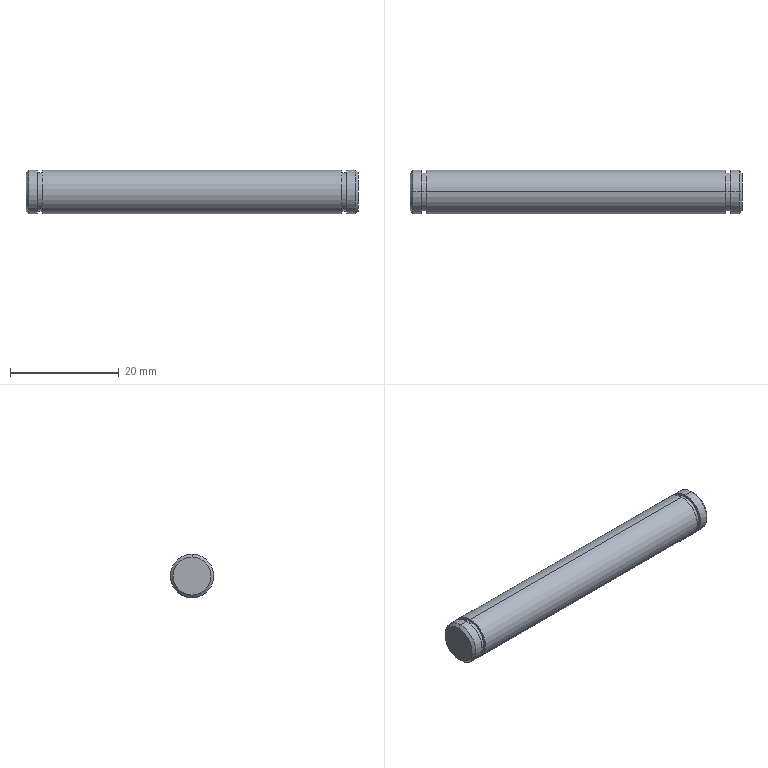Part | STEP file | 0217_Z_SCCG8-55-1 | 1 solid | 20 faces | box 61 x 8 x 8 mm | volume 3039 mm3 | cylinder 10 | plane 6 | cone 4 | commonest cylinder face diameters 8 x6 7 x4
STEP:
#1=CARTESIAN_POINT('',(0.,0.,0.));
#2=DIRECTION('',(0.,0.,1.));
#3=DIRECTION('',(1.,0.,0.));
#4=AXIS2_PLACEMENT_3D('',#1,#2,#3);
#5=CARTESIAN_POINT('',(3.,0.,-4.));
#6=VERTEX_POINT('',#5);
#7=CARTESIAN_POINT('',(3.,0.,4.));
#8=VERTEX_POINT('',#7);
#9=CARTESIAN_POINT('',(3.,0.,0.));
#10=DIRECTION('',(1.,0.,0.));
#11=DIRECTION('',(0.,0.,-1.));
#12=AXIS2_PLACEMENT_3D('',#9,#10,#11);
#13=CIRCLE('',#12,4.);
#14=CARTESIAN_POINT('',(30.5,0.,0.));
#15=DIRECTION('',(1.,0.,0.));
#16=DIRECTION('',(0.,0.,-1.));
#17=AXIS2_PLACEMENT_3D('',#14,#15,#16);
#18=CYLINDRICAL_SURFACE('',#17,4.);
#19=CARTESIAN_POINT('',(0.,-27.5));
#20=DIRECTION('',(1.,0.));
#21=VECTOR('',#20,1.);
#22=LINE('',#19,#21);
#23=(GEOMETRIC_REPRESENTATION_CONTEXT(2)PARAMETRIC_REPRESENTATION_CONTEXT()REPRESENTATION_CONTEXT('',''));
#24=DEFINITIONAL_REPRESENTATION('',(#22),#23);
#25=PCURVE('',#18,#24);
#26=CARTESIAN_POINT('',(3.,3.75,0.));
#27=DIRECTION('',(-1.,0.,0.));
#28=DIRECTION('',(0.,0.,1.));
#29=AXIS2_PLACEMENT_3D('',#26,#27,#28);
#30=PLANE('',#29);
#31=CARTESIAN_POINT('',(-4.,-3.75));
#32=CARTESIAN_POINT('',(-4.,3.178));
#33=CARTESIAN_POINT('',(2.,-0.2859));
#34=CARTESIAN_POINT('',(8.,-3.75));
#35=CARTESIAN_POINT('',(2.,-7.214));
#36=CARTESIAN_POINT('',(-4.,-10.678));
#37=CARTESIAN_POINT('',(-4.,-3.75));
#38=(BOUNDED_CURVE()B_SPLINE_CURVE(2,(#31,#32,#33,#34,#35,#36,#37),.UNSPECIFIED.,.T.,.F.)B_SPLINE_CURVE_WITH_KNOTS((1,2,2,2,2,1),(-2.094,0.,2.094,4.189,6.283,8.378),.UNSPECIFIED.)CURVE()GEOMETRIC_REPRESENTATION_ITEM()RATIONAL_B_SPLINE_CURVE((1.,0.5,1.,0.5,1.,0.5,1.))REPRESENTATION_ITEM(''));
#39=(GEOMETRIC_REPRESENTATION_CONTEXT(2)PARAMETRIC_REPRESENTATION_CONTEXT()REPRESENTATION_CONTEXT('',''));
#40=DEFINITIONAL_REPRESENTATION('',(#38),#39);
#41=PCURVE('',#30,#40);
#42=SURFACE_CURVE('',#13,(#25,#41),.PCURVE_S1.);
#43=EDGE_CURVE('',#6,#8,#42,.T.);
#44=ORIENTED_EDGE('',*,*,#43,.T.);
#45=CARTESIAN_POINT('',(58.,0.,4.));
#46=VERTEX_POINT('',#45);
#47=CARTESIAN_POINT('',(30.5,0.,4.));
#48=DIRECTION('',(1.,0.,0.));
#49=VECTOR('',#48,1.);
#50=LINE('',#47,#49);
#51=CARTESIAN_POINT('',(3.142,0.));
#52=DIRECTION('',(0.,1.));
#53=VECTOR('',#52,1.);
#54=LINE('',#51,#53);
#55=(GEOMETRIC_REPRESENTATION_CONTEXT(2)PARAMETRIC_REPRESENTATION_CONTEXT()REPRESENTATION_CONTEXT('',''));
#56=DEFINITIONAL_REPRESENTATION('',(#54),#55);
#57=PCURVE('',#18,#56);
#58=CARTESIAN_POINT('',(30.5,0.,0.));
#59=DIRECTION('',(1.,0.,0.));
#60=DIRECTION('',(0.,0.,-1.));
#61=AXIS2_PLACEMENT_3D('',#58,#59,#60);
#62=CYLINDRICAL_SURFACE('',#61,4.);
#63=CARTESIAN_POINT('',(3.142,0.));
#64=DIRECTION('',(0.,1.));
#65=VECTOR('',#64,1.);
#66=LINE('',#63,#65);
#67=(GEOMETRIC_REPRESENTATION_CONTEXT(2)PARAMETRIC_REPRESENTATION_CONTEXT()REPRESENTATION_CONTEXT('',''));
#68=DEFINITIONAL_REPRESENTATION('',(#66),#67);
#69=PCURVE('',#62,#68);
#70=SURFACE_CURVE('',#50,(#57,#69),.PCURVE_S1.);
#71=EDGE_CURVE('',#8,#46,#70,.T.);
#72=ORIENTED_EDGE('',*,*,#71,.T.);
#73=CARTESIAN_POINT('',(58.,0.,-4.));
#74=VERTEX_POINT('',#73);
#75=CARTESIAN_POINT('',(58.,0.,0.));
#76=DIRECTION('',(-1.,0.,0.));
#77=DIRECTION('',(0.,0.,-1.));
#78=AXIS2_PLACEMENT_3D('',#75,#76,#77);
#79=CIRCLE('',#78,4.);
#80=CARTESIAN_POINT('',(6.283,27.5));
#81=DIRECTION('',(-1.,0.));
#82=VECTOR('',#81,1.);
#83=LINE('',#80,#82);
#84=(GEOMETRIC_REPRESENTATION_CONTEXT(2)PARAMETRIC_REPRESENTATION_CONTEXT()REPRESENTATION_CONTEXT('',''));
#85=DEFINITIONAL_REPRESENTATION('',(#83),#84);
#86=PCURVE('',#18,#85);
#87=CARTESIAN_POINT('',(58.,3.75,0.));
#88=DIRECTION('',(1.,0.,0.));
#89=DIRECTION('',(0.,0.,-1.));
#90=AXIS2_PLACEMENT_3D('',#87,#88,#89);
#91=PLANE('',#90);
#92=CARTESIAN_POINT('',(4.,-3.75));
#93=CARTESIAN_POINT('',(4.,-10.678));
#94=CARTESIAN_POINT('',(-2.,-7.214));
#95=CARTESIAN_POINT('',(-8.,-3.75));
#96=CARTESIAN_POINT('',(-2.,-0.2859));
#97=CARTESIAN_POINT('',(4.,3.178));
#98=CARTESIAN_POINT('',(4.,-3.75));
#99=(BOUNDED_CURVE()B_SPLINE_CURVE(2,(#92,#93,#94,#95,#96,#97,#98),.UNSPECIFIED.,.T.,.F.)B_SPLINE_CURVE_WITH_KNOTS((1,2,2,2,2,1),(-2.094,0.,2.094,4.189,6.283,8.378),.UNSPECIFIED.)CURVE()GEOMETRIC_REPRESENTATION_ITEM()RATIONAL_B_SPLINE_CURVE((1.,0.5,1.,0.5,1.,0.5,1.))REPRESENTATION_ITEM(''));
#100=(GEOMETRIC_REPRESENTATION_CONTEXT(2)PARAMETRIC_REPRESENTATION_CONTEXT()REPRESENTATION_CONTEXT('',''));
#101=DEFINITIONAL_REPRESENTATION('',(#99),#100);
#102=PCURVE('',#91,#101);
#103=SURFACE_CURVE('',#79,(#86,#102),.PCURVE_S1.);
#104=EDGE_CURVE('',#46,#74,#103,.T.);
#105=ORIENTED_EDGE('',*,*,#104,.T.);
#106=CARTESIAN_POINT('',(30.5,0.,-4.));
#107=DIRECTION('',(1.,0.,0.));
#108=VECTOR('',#107,1.);
#109=LINE('',#106,#108);
#110=CARTESIAN_POINT('',(0.,0.));
#111=DIRECTION('',(0.,1.));
#112=VECTOR('',#111,1.);
#113=LINE('',#110,#112);
#114=(GEOMETRIC_REPRESENTATION_CONTEXT(2)PARAMETRIC_REPRESENTATION_CONTEXT()REPRESENTATION_CONTEXT('',''));
#115=DEFINITIONAL_REPRESENTATION('',(#113),#114);
#116=PCURVE('',#18,#115);
#117=CARTESIAN_POINT('',(6.283,0.));
#118=DIRECTION('',(0.,1.));
#119=VECTOR('',#118,1.);
#120=LINE('',#117,#119);
#121=(GEOMETRIC_REPRESENTATION_CONTEXT(2)PARAMETRIC_REPRESENTATION_CONTEXT()REPRESENTATION_CONTEXT('',''));
#122=DEFINITIONAL_REPRESENTATION('',(#120),#121);
#123=PCURVE('',#62,#122);
#124=SURFACE_CURVE('',#109,(#116,#123),.PCURVE_S1.);
#125=EDGE_CURVE('',#6,#74,#124,.T.);
#126=ORIENTED_EDGE('',*,*,#125,.F.);
#127=EDGE_LOOP('',(#44,#72,#105,#126));
#128=FACE_BOUND('',#127,.T.);
#129=ADVANCED_FACE('',(#128),#18,.T.);
#130=CARTESIAN_POINT('',(2.1,0.,-3.5));
#131=VERTEX_POINT('',#130);
#132=CARTESIAN_POINT('',(2.1,0.,3.5));
#133=VERTEX_POINT('',#132);
#134=CARTESIAN_POINT('',(2.1,0.,0.));
#135=DIRECTION('',(1.,0.,0.));
#136=DIRECTION('',(0.,0.,-1.));
#137=AXIS2_PLACEMENT_3D('',#134,#135,#136);
#138=CIRCLE('',#137,3.5);
#139=CARTESIAN_POINT('',(2.55,0.,0.));
#140=DIRECTION('',(1.,0.,0.));
#141=DIRECTION('',(0.,0.,-1.));
#142=AXIS2_PLACEMENT_3D('',#139,#140,#141);
#143=CYLINDRICAL_SURFACE('',#142,3.5);
#144=CARTESIAN_POINT('',(0.,-0.45));
#145=DIRECTION('',(1.,0.));
#146=VECTOR('',#145,1.);
#147=LINE('',#144,#146);
#148=(GEOMETRIC_REPRESENTATION_CONTEXT(2)PARAMETRIC_REPRESENTATION_CONTEXT()REPRESENTATION_CONTEXT('',''));
#149=DEFINITIONAL_REPRESENTATION('',(#147),#148);
#150=PCURVE('',#143,#149);
#151=CARTESIAN_POINT('',(2.1,3.75,0.));
#152=DIRECTION('',(1.,0.,0.));
#153=DIRECTION('',(0.,0.,-1.));
#154=AXIS2_PLACEMENT_3D('',#151,#152,#153);
#155=PLANE('',#154);
#156=CARTESIAN_POINT('',(0.,-3.75));
#157=DIRECTION('',(1.,0.));
#158=AXIS2_PLACEMENT_2D('',#156,#157);
#159=CIRCLE('',#158,3.5);
#160=(GEOMETRIC_REPRESENTATION_CONTEXT(2)PARAMETRIC_REPRESENTATION_CONTEXT()REPRESENTATION_CONTEXT('',''));
#161=DEFINITIONAL_REPRESENTATION('',(#159),#160);
#162=PCURVE('',#155,#161);
#163=SURFACE_CURVE('',#138,(#150,#162),.PCURVE_S1.);
#164=EDGE_CURVE('',#131,#133,#163,.T.);
#165=ORIENTED_EDGE('',*,*,#164,.T.);
#166=CARTESIAN_POINT('',(3.,0.,3.5));
#167=VERTEX_POINT('',#166);
#168=CARTESIAN_POINT('',(2.55,0.,3.5));
#169=DIRECTION('',(1.,0.,0.));
#170=VECTOR('',#169,1.);
#171=LINE('',#168,#170);
#172=CARTESIAN_POINT('',(3.142,0.));
#173=DIRECTION('',(0.,1.));
#174=VECTOR('',#173,1.);
#175=LINE('',#172,#174);
#176=(GEOMETRIC_REPRESENTATION_CONTEXT(2)PARAMETRIC_REPRESENTATION_CONTEXT()REPRESENTATION_CONTEXT('',''));
#177=DEFINITIONAL_REPRESENTATION('',(#175),#176);
#178=PCURVE('',#143,#177);
#179=CARTESIAN_POINT('',(2.55,0.,0.));
#180=DIRECTION('',(1.,0.,0.));
#181=DIRECTION('',(0.,0.,-1.));
#182=AXIS2_PLACEMENT_3D('',#179,#180,#181);
#183=CYLINDRICAL_SURFACE('',#182,3.5);
#184=CARTESIAN_POINT('',(3.142,0.));
#185=DIRECTION('',(0.,1.));
#186=VECTOR('',#185,1.);
#187=LINE('',#184,#186);
#188=(GEOMETRIC_REPRESENTATION_CONTEXT(2)PARAMETRIC_REPRESENTATION_CONTEXT()REPRESENTATION_CONTEXT('',''));
#189=DEFINITIONAL_REPRESENTATION('',(#187),#188);
#190=PCURVE('',#183,#189);
#191=SURFACE_CURVE('',#171,(#178,#190),.PCURVE_S1.);
#192=EDGE_CURVE('',#133,#167,#191,.T.);
#193=ORIENTED_EDGE('',*,*,#192,.T.);
#194=CARTESIAN_POINT('',(3.,0.,-3.5));
#195=VERTEX_POINT('',#194);
#196=CARTESIAN_POINT('',(3.,0.,0.));
#197=DIRECTION('',(1.,0.,0.));
#198=DIRECTION('',(0.,0.,-1.));
#199=AXIS2_PLACEMENT_3D('',#196,#197,#198);
#200=CIRCLE('',#199,3.5);
#201=CARTESIAN_POINT('',(0.,0.45));
#202=DIRECTION('',(1.,0.));
#203=VECTOR('',#202,1.);
#204=LINE('',#201,#203);
#205=(GEOMETRIC_REPRESENTATION_CONTEXT(2)PARAMETRIC_REPRESENTATION_CONTEXT()REPRESENTATION_CONTEXT('',''));
#206=DEFINITIONAL_REPRESENTATION('',(#204),#205);
#207=PCURVE('',#143,#206);
#208=CARTESIAN_POINT('',(-3.5,-3.75));
#209=CARTESIAN_POINT('',(-3.5,2.312));
#210=CARTESIAN_POINT('',(1.75,-0.7189));
#211=CARTESIAN_POINT('',(7.,-3.75));
#212=CARTESIAN_POINT('',(1.75,-6.781));
#213=CARTESIAN_POINT('',(-3.5,-9.812));
#214=CARTESIAN_POINT('',(-3.5,-3.75));
#215=(BOUNDED_CURVE()B_SPLINE_CURVE(2,(#208,#209,#210,#211,#212,#213,#214),.UNSPECIFIED.,.T.,.F.)B_SPLINE_CURVE_WITH_KNOTS((1,2,2,2,2,1),(-2.094,0.,2.094,4.189,6.283,8.378),.UNSPECIFIED.)CURVE()GEOMETRIC_REPRESENTATION_ITEM()RATIONAL_B_SPLINE_CURVE((1.,0.5,1.,0.5,1.,0.5,1.))REPRESENTATION_ITEM(''));
#216=(GEOMETRIC_REPRESENTATION_CONTEXT(2)PARAMETRIC_REPRESENTATION_CONTEXT()REPRESENTATION_CONTEXT('',''));
#217=DEFINITIONAL_REPRESENTATION('',(#215),#216);
#218=PCURVE('',#30,#217);
#219=SURFACE_CURVE('',#200,(#207,#218),.PCURVE_S1.);
#220=EDGE_CURVE('',#195,#167,#219,.T.);
#221=ORIENTED_EDGE('',*,*,#220,.F.);
#222=CARTESIAN_POINT('',(2.55,0.,-3.5));
#223=DIRECTION('',(1.,0.,0.));
#224=VECTOR('',#223,1.);
#225=LINE('',#222,#224);
#226=CARTESIAN_POINT('',(0.,0.));
#227=DIRECTION('',(0.,1.));
#228=VECTOR('',#227,1.);
#229=LINE('',#226,#228);
#230=(GEOMETRIC_REPRESENTATION_CONTEXT(2)PARAMETRIC_REPRESENTATION_CONTEXT()REPRESENTATION_CONTEXT('',''));
#231=DEFINITIONAL_REPRESENTATION('',(#229),#230);
#232=PCURVE('',#143,#231);
#233=CARTESIAN_POINT('',(6.283,0.));
#234=DIRECTION('',(0.,1.));
#235=VECTOR('',#234,1.);
#236=LINE('',#233,#235);
#237=(GEOMETRIC_REPRESENTATION_CONTEXT(2)PARAMETRIC_REPRESENTATION_CONTEXT()REPRESENTATION_CONTEXT('',''));
#238=DEFINITIONAL_REPRESENTATION('',(#236),#237);
#239=PCURVE('',#183,#238);
#240=SURFACE_CURVE('',#225,(#232,#239),.PCURVE_S1.);
#241=EDGE_CURVE('',#131,#195,#240,.T.);
#242=ORIENTED_EDGE('',*,*,#241,.F.);
#243=EDGE_LOOP('',(#165,#193,#221,#242));
#244=FACE_BOUND('',#243,.T.);
#245=ADVANCED_FACE('',(#244),#143,.T.);
#246=CARTESIAN_POINT('',(58.,0.,3.5));
#247=VERTEX_POINT('',#246);
#248=CARTESIAN_POINT('',(58.,0.,-3.5));
#249=VERTEX_POINT('',#248);
#250=CARTESIAN_POINT('',(58.,0.,0.));
#251=DIRECTION('',(-1.,0.,0.));
#252=DIRECTION('',(0.,0.,-1.));
#253=AXIS2_PLACEMENT_3D('',#250,#251,#252);
#254=CIRCLE('',#253,3.5);
#255=CARTESIAN_POINT('',(58.45,0.,0.));
#256=DIRECTION('',(1.,0.,0.));
#257=DIRECTION('',(0.,0.,-1.));
#258=AXIS2_PLACEMENT_3D('',#255,#256,#257);
#259=CYLINDRICAL_SURFACE('',#258,3.5);
#260=CARTESIAN_POINT('',(6.283,-0.45));
#261=DIRECTION('',(-1.,0.));
#262=VECTOR('',#261,1.);
#263=LINE('',#260,#262);
#264=(GEOMETRIC_REPRESENTATION_CONTEXT(2)PARAMETRIC_REPRESENTATION_CONTEXT()REPRESENTATION_CONTEXT('',''));
#265=DEFINITIONAL_REPRESENTATION('',(#263),#264);
#266=PCURVE('',#259,#265);
#267=CARTESIAN_POINT('',(3.5,-3.75));
#268=CARTESIAN_POINT('',(3.5,-9.812));
#269=CARTESIAN_POINT('',(-1.75,-6.781));
#270=CARTESIAN_POINT('',(-7.,-3.75));
#271=CARTESIAN_POINT('',(-1.75,-0.7189));
#272=CARTESIAN_POINT('',(3.5,2.312));
#273=CARTESIAN_POINT('',(3.5,-3.75));
#274=(BOUNDED_CURVE()B_SPLINE_CURVE(2,(#267,#268,#269,#270,#271,#272,#273),.UNSPECIFIED.,.T.,.F.)B_SPLINE_CURVE_WITH_KNOTS((1,2,2,2,2,1),(-2.094,0.,2.094,4.189,6.283,8.378),.UNSPECIFIED.)CURVE()GEOMETRIC_REPRESENTATION_ITEM()RATIONAL_B_SPLINE_CURVE((1.,0.5,1.,0.5,1.,0.5,1.))REPRESENTATION_ITEM(''));
#275=(GEOMETRIC_REPRESENTATION_CONTEXT(2)PARAMETRIC_REPRESENTATION_CONTEXT()REPRESENTATION_CONTEXT('',''));
#276=DEFINITIONAL_REPRESENTATION('',(#274),#275);
#277=PCURVE('',#91,#276);
#278=SURFACE_CURVE('',#254,(#266,#277),.PCURVE_S1.);
#279=EDGE_CURVE('',#247,#249,#278,.T.);
#280=ORIENTED_EDGE('',*,*,#279,.F.);
#281=CARTESIAN_POINT('',(58.9,0.,3.5));
#282=VERTEX_POINT('',#281);
#283=CARTESIAN_POINT('',(58.45,0.,3.5));
#284=DIRECTION('',(1.,0.,0.));
#285=VECTOR('',#284,1.);
#286=LINE('',#283,#285);
#287=CARTESIAN_POINT('',(3.142,0.));
#288=DIRECTION('',(0.,1.));
#289=VECTOR('',#288,1.);
#290=LINE('',#287,#289);
#291=(GEOMETRIC_REPRESENTATION_CONTEXT(2)PARAMETRIC_REPRESENTATION_CONTEXT()REPRESENTATION_CONTEXT('',''));
#292=DEFINITIONAL_REPRESENTATION('',(#290),#291);
#293=PCURVE('',#259,#292);
#294=CARTESIAN_POINT('',(58.45,0.,0.));
#295=DIRECTION('',(1.,0.,0.));
#296=DIRECTION('',(0.,0.,-1.));
#297=AXIS2_PLACEMENT_3D('',#294,#295,#296);
#298=CYLINDRICAL_SURFACE('',#297,3.5);
#299=CARTESIAN_POINT('',(3.142,0.));
#300=DIRECTION('',(0.,1.));
#301=VECTOR('',#300,1.);
#302=LINE('',#299,#301);
#303=(GEOMETRIC_REPRESENTATION_CONTEXT(2)PARAMETRIC_REPRESENTATION_CONTEXT()REPRESENTATION_CONTEXT('',''));
#304=DEFINITIONAL_REPRESENTATION('',(#302),#303);
#305=PCURVE('',#298,#304);
#306=SURFACE_CURVE('',#286,(#293,#305),.PCURVE_S1.);
#307=EDGE_CURVE('',#247,#282,#306,.T.);
#308=ORIENTED_EDGE('',*,*,#307,.T.);
#309=CARTESIAN_POINT('',(58.9,0.,-3.5));
#310=VERTEX_POINT('',#309);
#311=CARTESIAN_POINT('',(58.9,0.,0.));
#312=DIRECTION('',(-1.,0.,0.));
#313=DIRECTION('',(0.,0.,-1.));
#314=AXIS2_PLACEMENT_3D('',#311,#312,#313);
#315=CIRCLE('',#314,3.5);
#316=CARTESIAN_POINT('',(6.283,0.45));
#317=DIRECTION('',(-1.,0.));
#318=VECTOR('',#317,1.);
#319=LINE('',#316,#318);
#320=(GEOMETRIC_REPRESENTATION_CONTEXT(2)PARAMETRIC_REPRESENTATION_CONTEXT()REPRESENTATION_CONTEXT('',''));
#321=DEFINITIONAL_REPRESENTATION('',(#319),#320);
#322=PCURVE('',#259,#321);
#323=CARTESIAN_POINT('',(58.9,3.75,0.));
#324=DIRECTION('',(-1.,0.,0.));
#325=DIRECTION('',(0.,0.,1.));
#326=AXIS2_PLACEMENT_3D('',#323,#324,#325);
#327=PLANE('',#326);
#328=CARTESIAN_POINT('',(0.,-3.75));
#329=DIRECTION('',(-1.,0.));
#330=AXIS2_PLACEMENT_2D('',#328,#329);
#331=CIRCLE('',#330,3.5);
#332=(GEOMETRIC_REPRESENTATION_CONTEXT(2)PARAMETRIC_REPRESENTATION_CONTEXT()REPRESENTATION_CONTEXT('',''));
#333=DEFINITIONAL_REPRESENTATION('',(#331),#332);
#334=PCURVE('',#327,#333);
#335=SURFACE_CURVE('',#315,(#322,#334),.PCURVE_S1.);
#336=EDGE_CURVE('',#282,#310,#335,.T.);
#337=ORIENTED_EDGE('',*,*,#336,.T.);
#338=CARTESIAN_POINT('',(58.45,0.,-3.5));
#339=DIRECTION('',(1.,0.,0.));
#340=VECTOR('',#339,1.);
#341=LINE('',#338,#340);
#342=CARTESIAN_POINT('',(0.,0.));
#343=DIRECTION('',(0.,1.));
#344=VECTOR('',#343,1.);
#345=LINE('',#342,#344);
#346=(GEOMETRIC_REPRESENTATION_CONTEXT(2)PARAMETRIC_REPRESENTATION_CONTEXT()REPRESENTATION_CONTEXT('',''));
#347=DEFINITIONAL_REPRESENTATION('',(#345),#346);
#348=PCURVE('',#259,#347);
#349=CARTESIAN_POINT('',(6.283,0.));
#350=DIRECTION('',(0.,1.));
#351=VECTOR('',#350,1.);
#352=LINE('',#349,#351);
#353=(GEOMETRIC_REPRESENTATION_CONTEXT(2)PARAMETRIC_REPRESENTATION_CONTEXT()REPRESENTATION_CONTEXT('',''));
#354=DEFINITIONAL_REPRESENTATION('',(#352),#353);
#355=PCURVE('',#298,#354);
#356=SURFACE_CURVE('',#341,(#348,#355),.PCURVE_S1.);
#357=EDGE_CURVE('',#249,#310,#356,.T.);
#358=ORIENTED_EDGE('',*,*,#357,.F.);
#359=EDGE_LOOP('',(#280,#308,#337,#358));
#360=FACE_BOUND('',#359,.T.);
#361=ADVANCED_FACE('',(#360),#259,.T.);
#362=CARTESIAN_POINT('',(0.5,0.,-4.));
#363=VERTEX_POINT('',#362);
#364=CARTESIAN_POINT('',(0.5,0.,4.));
#365=VERTEX_POINT('',#364);
#366=CARTESIAN_POINT('',(0.5,0.,0.));
#367=DIRECTION('',(1.,0.,0.));
#368=DIRECTION('',(0.,0.,-1.));
#369=AXIS2_PLACEMENT_3D('',#366,#367,#368);
#370=CIRCLE('',#369,4.);
#371=CARTESIAN_POINT('',(1.3,0.,0.));
#372=DIRECTION('',(1.,0.,0.));
#373=DIRECTION('',(0.,0.,-1.));
#374=AXIS2_PLACEMENT_3D('',#371,#372,#373);
#375=CYLINDRICAL_SURFACE('',#374,4.);
#376=CARTESIAN_POINT('',(0.,-0.8));
#377=DIRECTION('',(1.,0.));
#378=VECTOR('',#377,1.);
#379=LINE('',#376,#378);
#380=(GEOMETRIC_REPRESENTATION_CONTEXT(2)PARAMETRIC_REPRESENTATION_CONTEXT()REPRESENTATION_CONTEXT('',''));
#381=DEFINITIONAL_REPRESENTATION('',(#379),#380);
#382=PCURVE('',#375,#381);
#383=CARTESIAN_POINT('',(0.5,0.,0.));
#384=DIRECTION('',(1.,0.,0.));
#385=DIRECTION('',(0.,0.,-1.));
#386=AXIS2_PLACEMENT_3D('',#383,#384,#385);
#387=CONICAL_SURFACE('',#386,4.,0.7854);
#388=CARTESIAN_POINT('',(0.,0.));
#389=DIRECTION('',(1.,0.));
#390=VECTOR('',#389,1.);
#391=LINE('',#388,#390);
#392=(GEOMETRIC_REPRESENTATION_CONTEXT(2)PARAMETRIC_REPRESENTATION_CONTEXT()REPRESENTATION_CONTEXT('',''));
#393=DEFINITIONAL_REPRESENTATION('',(#391),#392);
#394=PCURVE('',#387,#393);
#395=SURFACE_CURVE('',#370,(#382,#394),.PCURVE_S1.);
#396=EDGE_CURVE('',#363,#365,#395,.T.);
#397=ORIENTED_EDGE('',*,*,#396,.T.);
#398=CARTESIAN_POINT('',(2.1,0.,4.));
#399=VERTEX_POINT('',#398);
#400=CARTESIAN_POINT('',(1.3,0.,4.));
#401=DIRECTION('',(1.,0.,0.));
#402=VECTOR('',#401,1.);
#403=LINE('',#400,#402);
#404=CARTESIAN_POINT('',(3.142,0.));
#405=DIRECTION('',(0.,1.));
#406=VECTOR('',#405,1.);
#407=LINE('',#404,#406);
#408=(GEOMETRIC_REPRESENTATION_CONTEXT(2)PARAMETRIC_REPRESENTATION_CONTEXT()REPRESENTATION_CONTEXT('',''));
#409=DEFINITIONAL_REPRESENTATION('',(#407),#408);
#410=PCURVE('',#375,#409);
#411=CARTESIAN_POINT('',(1.3,0.,0.));
#412=DIRECTION('',(1.,0.,0.));
#413=DIRECTION('',(0.,0.,-1.));
#414=AXIS2_PLACEMENT_3D('',#411,#412,#413);
#415=CYLINDRICAL_SURFACE('',#414,4.);
#416=CARTESIAN_POINT('',(3.142,0.));
#417=DIRECTION('',(0.,1.));
#418=VECTOR('',#417,1.);
#419=LINE('',#416,#418);
#420=(GEOMETRIC_REPRESENTATION_CONTEXT(2)PARAMETRIC_REPRESENTATION_CONTEXT()REPRESENTATION_CONTEXT('',''));
#421=DEFINITIONAL_REPRESENTATION('',(#419),#420);
#422=PCURVE('',#415,#421);
#423=SURFACE_CURVE('',#403,(#410,#422),.PCURVE_S1.);
#424=EDGE_CURVE('',#365,#399,#423,.T.);
#425=ORIENTED_EDGE('',*,*,#424,.T.);
#426=CARTESIAN_POINT('',(2.1,0.,-4.));
#427=VERTEX_POINT('',#426);
#428=CARTESIAN_POINT('',(2.1,0.,0.));
#429=DIRECTION('',(1.,0.,0.));
#430=DIRECTION('',(0.,0.,-1.));
#431=AXIS2_PLACEMENT_3D('',#428,#429,#430);
#432=CIRCLE('',#431,4.);
#433=CARTESIAN_POINT('',(0.,0.8));
#434=DIRECTION('',(1.,0.));
#435=VECTOR('',#434,1.);
#436=LINE('',#433,#435);
#437=(GEOMETRIC_REPRESENTATION_CONTEXT(2)PARAMETRIC_REPRESENTATION_CONTEXT()REPRESENTATION_CONTEXT('',''));
#438=DEFINITIONAL_REPRESENTATION('',(#436),#437);
#439=PCURVE('',#375,#438);
#440=CARTESIAN_POINT('',(0.,-3.75));
#441=DIRECTION('',(1.,0.));
#442=AXIS2_PLACEMENT_2D('',#440,#441);
#443=CIRCLE('',#442,4.);
#444=(GEOMETRIC_REPRESENTATION_CONTEXT(2)PARAMETRIC_REPRESENTATION_CONTEXT()REPRESENTATION_CONTEXT('',''));
#445=DEFINITIONAL_REPRESENTATION('',(#443),#444);
#446=PCURVE('',#155,#445);
#447=SURFACE_CURVE('',#432,(#439,#446),.PCURVE_S1.);
#448=EDGE_CURVE('',#427,#399,#447,.T.);
#449=ORIENTED_EDGE('',*,*,#448,.F.);
#450=CARTESIAN_POINT('',(1.3,0.,-4.));
#451=DIRECTION('',(1.,0.,0.));
#452=VECTOR('',#451,1.);
#453=LINE('',#450,#452);
#454=CARTESIAN_POINT('',(0.,0.));
#455=DIRECTION('',(0.,1.));
#456=VECTOR('',#455,1.);
#457=LINE('',#454,#456);
#458=(GEOMETRIC_REPRESENTATION_CONTEXT(2)PARAMETRIC_REPRESENTATION_CONTEXT()REPRESENTATION_CONTEXT('',''));
#459=DEFINITIONAL_REPRESENTATION('',(#457),#458);
#460=PCURVE('',#375,#459);
#461=CARTESIAN_POINT('',(6.283,0.));
#462=DIRECTION('',(0.,1.));
#463=VECTOR('',#462,1.);
#464=LINE('',#461,#463);
#465=(GEOMETRIC_REPRESENTATION_CONTEXT(2)PARAMETRIC_REPRESENTATION_CONTEXT()REPRESENTATION_CONTEXT('',''));
#466=DEFINITIONAL_REPRESENTATION('',(#464),#465);
#467=PCURVE('',#415,#466);
#468=SURFACE_CURVE('',#453,(#460,#467),.PCURVE_S1.);
#469=EDGE_CURVE('',#363,#427,#468,.T.);
#470=ORIENTED_EDGE('',*,*,#469,.F.);
#471=EDGE_LOOP('',(#397,#425,#449,#470));
#472=FACE_BOUND('',#471,.T.);
#473=ADVANCED_FACE('',(#472),#375,.T.);
#474=CARTESIAN_POINT('',(58.9,0.,4.));
#475=VERTEX_POINT('',#474);
#476=CARTESIAN_POINT('',(58.9,0.,-4.));
#477=VERTEX_POINT('',#476);
#478=CARTESIAN_POINT('',(58.9,0.,0.));
#479=DIRECTION('',(-1.,0.,0.));
#480=DIRECTION('',(0.,0.,-1.));
#481=AXIS2_PLACEMENT_3D('',#478,#479,#480);
#482=CIRCLE('',#481,4.);
#483=CARTESIAN_POINT('',(59.7,0.,0.));
#484=DIRECTION('',(1.,0.,0.));
#485=DIRECTION('',(0.,0.,-1.));
#486=AXIS2_PLACEMENT_3D('',#483,#484,#485);
#487=CYLINDRICAL_SURFACE('',#486,4.);
#488=CARTESIAN_POINT('',(6.283,-0.8));
#489=DIRECTION('',(-1.,0.));
#490=VECTOR('',#489,1.);
#491=LINE('',#488,#490);
#492=(GEOMETRIC_REPRESENTATION_CONTEXT(2)PARAMETRIC_REPRESENTATION_CONTEXT()REPRESENTATION_CONTEXT('',''));
#493=DEFINITIONAL_REPRESENTATION('',(#491),#492);
#494=PCURVE('',#487,#493);
#495=CARTESIAN_POINT('',(0.,-3.75));
#496=DIRECTION('',(-1.,0.));
#497=AXIS2_PLACEMENT_2D('',#495,#496);
#498=CIRCLE('',#497,4.);
#499=(GEOMETRIC_REPRESENTATION_CONTEXT(2)PARAMETRIC_REPRESENTATION_CONTEXT()REPRESENTATION_CONTEXT('',''));
#500=DEFINITIONAL_REPRESENTATION('',(#498),#499);
#501=PCURVE('',#327,#500);
#502=SURFACE_CURVE('',#482,(#494,#501),.PCURVE_S1.);
#503=EDGE_CURVE('',#475,#477,#502,.T.);
#504=ORIENTED_EDGE('',*,*,#503,.F.);
#505=CARTESIAN_POINT('',(60.5,0.,4.));
#506=VERTEX_POINT('',#505);
#507=CARTESIAN_POINT('',(59.7,0.,4.));
#508=DIRECTION('',(1.,0.,0.));
#509=VECTOR('',#508,1.);
#510=LINE('',#507,#509);
#511=CARTESIAN_POINT('',(3.142,0.));
#512=DIRECTION('',(0.,1.));
#513=VECTOR('',#512,1.);
#514=LINE('',#511,#513);
#515=(GEOMETRIC_REPRESENTATION_CONTEXT(2)PARAMETRIC_REPRESENTATION_CONTEXT()REPRESENTATION_CONTEXT('',''));
#516=DEFINITIONAL_REPRESENTATION('',(#514),#515);
#517=PCURVE('',#487,#516);
#518=CARTESIAN_POINT('',(59.7,0.,0.));
#519=DIRECTION('',(1.,0.,0.));
#520=DIRECTION('',(0.,0.,-1.));
#521=AXIS2_PLACEMENT_3D('',#518,#519,#520);
#522=CYLINDRICAL_SURFACE('',#521,4.);
#523=CARTESIAN_POINT('',(3.142,0.));
#524=DIRECTION('',(0.,1.));
#525=VECTOR('',#524,1.);
#526=LINE('',#523,#525);
#527=(GEOMETRIC_REPRESENTATION_CONTEXT(2)PARAMETRIC_REPRESENTATION_CONTEXT()REPRESENTATION_CONTEXT('',''));
#528=DEFINITIONAL_REPRESENTATION('',(#526),#527);
#529=PCURVE('',#522,#528);
#530=SURFACE_CURVE('',#510,(#517,#529),.PCURVE_S1.);
#531=EDGE_CURVE('',#475,#506,#530,.T.);
#532=ORIENTED_EDGE('',*,*,#531,.T.);
#533=CARTESIAN_POINT('',(60.5,0.,-4.));
#534=VERTEX_POINT('',#533);
#535=CARTESIAN_POINT('',(60.5,0.,0.));
#536=DIRECTION('',(-1.,0.,0.));
#537=DIRECTION('',(0.,0.,-1.));
#538=AXIS2_PLACEMENT_3D('',#535,#536,#537);
#539=CIRCLE('',#538,4.);
#540=CARTESIAN_POINT('',(6.283,0.8));
#541=DIRECTION('',(-1.,0.));
#542=VECTOR('',#541,1.);
#543=LINE('',#540,#542);
#544=(GEOMETRIC_REPRESENTATION_CONTEXT(2)PARAMETRIC_REPRESENTATION_CONTEXT()REPRESENTATION_CONTEXT('',''));
#545=DEFINITIONAL_REPRESENTATION('',(#543),#544);
#546=PCURVE('',#487,#545);
#547=CARTESIAN_POINT('',(60.5,0.,0.));
#548=DIRECTION('',(-1.,0.,0.));
#549=DIRECTION('',(0.,0.,1.));
#550=AXIS2_PLACEMENT_3D('',#547,#548,#549);
#551=CONICAL_SURFACE('',#550,4.,0.7854);
#552=CARTESIAN_POINT('',(-3.142,0.));
#553=DIRECTION('',(1.,0.));
#554=VECTOR('',#553,1.);
#555=LINE('',#552,#554);
#556=(GEOMETRIC_REPRESENTATION_CONTEXT(2)PARAMETRIC_REPRESENTATION_CONTEXT()REPRESENTATION_CONTEXT('',''));
#557=DEFINITIONAL_REPRESENTATION('',(#555),#556);
#558=PCURVE('',#551,#557);
#559=SURFACE_CURVE('',#539,(#546,#558),.PCURVE_S1.);
#560=EDGE_CURVE('',#506,#534,#559,.T.);
#561=ORIENTED_EDGE('',*,*,#560,.T.);
#562=CARTESIAN_POINT('',(59.7,0.,-4.));
#563=DIRECTION('',(1.,0.,0.));
#564=VECTOR('',#563,1.);
#565=LINE('',#562,#564);
#566=CARTESIAN_POINT('',(0.,0.));
#567=DIRECTION('',(0.,1.));
#568=VECTOR('',#567,1.);
#569=LINE('',#566,#568);
#570=(GEOMETRIC_REPRESENTATION_CONTEXT(2)PARAMETRIC_REPRESENTATION_CONTEXT()REPRESENTATION_CONTEXT('',''));
#571=DEFINITIONAL_REPRESENTATION('',(#569),#570);
#572=PCURVE('',#487,#571);
#573=CARTESIAN_POINT('',(6.283,0.));
#574=DIRECTION('',(0.,1.));
#575=VECTOR('',#574,1.);
#576=LINE('',#573,#575);
#577=(GEOMETRIC_REPRESENTATION_CONTEXT(2)PARAMETRIC_REPRESENTATION_CONTEXT()REPRESENTATION_CONTEXT('',''));
#578=DEFINITIONAL_REPRESENTATION('',(#576),#577);
#579=PCURVE('',#522,#578);
#580=SURFACE_CURVE('',#565,(#572,#579),.PCURVE_S1.);
#581=EDGE_CURVE('',#477,#534,#580,.T.);
#582=ORIENTED_EDGE('',*,*,#581,.F.);
#583=EDGE_LOOP('',(#504,#532,#561,#582));
#584=FACE_BOUND('',#583,.T.);
#585=ADVANCED_FACE('',(#584),#487,.T.);
#586=CARTESIAN_POINT('',(0.,0.,-3.5));
#587=VERTEX_POINT('',#586);
#588=CARTESIAN_POINT('',(0.,0.,3.5));
#589=VERTEX_POINT('',#588);
#590=CARTESIAN_POINT('',(0.,0.,0.));
#591=DIRECTION('',(1.,0.,0.));
#592=DIRECTION('',(0.,0.,-1.));
#593=AXIS2_PLACEMENT_3D('',#590,#591,#592);
#594=CIRCLE('',#593,3.5);
#595=CARTESIAN_POINT('',(0.,-0.5));
#596=DIRECTION('',(1.,0.));
#597=VECTOR('',#596,1.);
#598=LINE('',#595,#597);
#599=(GEOMETRIC_REPRESENTATION_CONTEXT(2)PARAMETRIC_REPRESENTATION_CONTEXT()REPRESENTATION_CONTEXT('',''));
#600=DEFINITIONAL_REPRESENTATION('',(#598),#599);
#601=PCURVE('',#387,#600);
#602=CARTESIAN_POINT('',(0.,1.75,0.));
#603=DIRECTION('',(-1.,0.,0.));
#604=DIRECTION('',(0.,0.,1.));
#605=AXIS2_PLACEMENT_3D('',#602,#603,#604);
#606=PLANE('',#605);
#607=CARTESIAN_POINT('',(-3.5,-1.75));
#608=CARTESIAN_POINT('',(-3.5,4.312));
#609=CARTESIAN_POINT('',(1.75,1.281));
#610=CARTESIAN_POINT('',(7.,-1.75));
#611=CARTESIAN_POINT('',(1.75,-4.781));
#612=CARTESIAN_POINT('',(-3.5,-7.812));
#613=CARTESIAN_POINT('',(-3.5,-1.75));
#614=(BOUNDED_CURVE()B_SPLINE_CURVE(2,(#607,#608,#609,#610,#611,#612,#613),.UNSPECIFIED.,.T.,.F.)B_SPLINE_CURVE_WITH_KNOTS((1,2,2,2,2,1),(-2.094,0.,2.094,4.189,6.283,8.378),.UNSPECIFIED.)CURVE()GEOMETRIC_REPRESENTATION_ITEM()RATIONAL_B_SPLINE_CURVE((1.,0.5,1.,0.5,1.,0.5,1.))REPRESENTATION_ITEM(''));
#615=(GEOMETRIC_REPRESENTATION_CONTEXT(2)PARAMETRIC_REPRESENTATION_CONTEXT()REPRESENTATION_CONTEXT('',''));
#616=DEFINITIONAL_REPRESENTATION('',(#614),#615);
#617=PCURVE('',#606,#616);
#618=SURFACE_CURVE('',#594,(#601,#617),.PCURVE_S1.);
#619=EDGE_CURVE('',#587,#589,#618,.T.);
#620=ORIENTED_EDGE('',*,*,#619,.T.);
#621=CARTESIAN_POINT('',(0.5,0.,4.));
#622=DIRECTION('',(0.7071,0.,0.7071));
#623=VECTOR('',#622,1.);
#624=LINE('',#621,#623);
#625=CARTESIAN_POINT('',(3.142,0.));
#626=DIRECTION('',(0.,1.));
#627=VECTOR('',#626,1.);
#628=LINE('',#625,#627);
#629=(GEOMETRIC_REPRESENTATION_CONTEXT(2)PARAMETRIC_REPRESENTATION_CONTEXT()REPRESENTATION_CONTEXT('',''));
#630=DEFINITIONAL_REPRESENTATION('',(#628),#629);
#631=PCURVE('',#387,#630);
#632=CARTESIAN_POINT('',(0.5,0.,0.));
#633=DIRECTION('',(1.,0.,0.));
#634=DIRECTION('',(0.,0.,-1.));
#635=AXIS2_PLACEMENT_3D('',#632,#633,#634);
#636=CONICAL_SURFACE('',#635,4.,0.7854);
#637=CARTESIAN_POINT('',(3.142,0.));
#638=DIRECTION('',(0.,1.));
#639=VECTOR('',#638,1.);
#640=LINE('',#637,#639);
#641=(GEOMETRIC_REPRESENTATION_CONTEXT(2)PARAMETRIC_REPRESENTATION_CONTEXT()REPRESENTATION_CONTEXT('',''));
#642=DEFINITIONAL_REPRESENTATION('',(#640),#641);
#643=PCURVE('',#636,#642);
#644=SURFACE_CURVE('',#624,(#631,#643),.PCURVE_S1.);
#645=EDGE_CURVE('',#589,#365,#644,.T.);
#646=ORIENTED_EDGE('',*,*,#645,.T.);
#647=ORIENTED_EDGE('',*,*,#396,.F.);
#648=CARTESIAN_POINT('',(0.5,0.,-4.));
#649=DIRECTION('',(0.7071,0.,-0.7071));
#650=VECTOR('',#649,1.);
#651=LINE('',#648,#650);
#652=CARTESIAN_POINT('',(0.,0.));
#653=DIRECTION('',(0.,1.));
#654=VECTOR('',#653,1.);
#655=LINE('',#652,#654);
#656=(GEOMETRIC_REPRESENTATION_CONTEXT(2)PARAMETRIC_REPRESENTATION_CONTEXT()REPRESENTATION_CONTEXT('',''));
#657=DEFINITIONAL_REPRESENTATION('',(#655),#656);
#658=PCURVE('',#387,#657);
#659=CARTESIAN_POINT('',(6.283,0.));
#660=DIRECTION('',(0.,1.));
#661=VECTOR('',#660,1.);
#662=LINE('',#659,#661);
#663=(GEOMETRIC_REPRESENTATION_CONTEXT(2)PARAMETRIC_REPRESENTATION_CONTEXT()REPRESENTATION_CONTEXT('',''));
#664=DEFINITIONAL_REPRESENTATION('',(#662),#663);
#665=PCURVE('',#636,#664);
#666=SURFACE_CURVE('',#651,(#658,#665),.PCURVE_S1.);
#667=EDGE_CURVE('',#587,#363,#666,.T.);
#668=ORIENTED_EDGE('',*,*,#667,.F.);
#669=EDGE_LOOP('',(#620,#646,#647,#668));
#670=FACE_BOUND('',#669,.T.);
#671=ADVANCED_FACE('',(#670),#387,.T.);
#672=CARTESIAN_POINT('',(61.,0.,3.5));
#673=VERTEX_POINT('',#672);
#674=CARTESIAN_POINT('',(61.,0.,-3.5));
#675=VERTEX_POINT('',#674);
#676=CARTESIAN_POINT('',(61.,0.,0.));
#677=DIRECTION('',(-1.,0.,0.));
#678=DIRECTION('',(0.,0.,1.));
#679=AXIS2_PLACEMENT_3D('',#676,#677,#678);
#680=CIRCLE('',#679,3.5);
#681=CARTESIAN_POINT('',(0.,-0.5));
#682=DIRECTION('',(1.,0.));
#683=VECTOR('',#682,1.);
#684=LINE('',#681,#683);
#685=(GEOMETRIC_REPRESENTATION_CONTEXT(2)PARAMETRIC_REPRESENTATION_CONTEXT()REPRESENTATION_CONTEXT('',''));
#686=DEFINITIONAL_REPRESENTATION('',(#684),#685);
#687=PCURVE('',#551,#686);
#688=CARTESIAN_POINT('',(61.,1.75,0.));
#689=DIRECTION('',(1.,0.,0.));
#690=DIRECTION('',(0.,0.,-1.));
#691=AXIS2_PLACEMENT_3D('',#688,#689,#690);
#692=PLANE('',#691);
#693=CARTESIAN_POINT('',(-3.5,-1.75));
#694=CARTESIAN_POINT('',(-3.5,4.312));
#695=CARTESIAN_POINT('',(1.75,1.281));
#696=CARTESIAN_POINT('',(7.,-1.75));
#697=CARTESIAN_POINT('',(1.75,-4.781));
#698=CARTESIAN_POINT('',(-3.5,-7.812));
#699=CARTESIAN_POINT('',(-3.5,-1.75));
#700=(BOUNDED_CURVE()B_SPLINE_CURVE(2,(#693,#694,#695,#696,#697,#698,#699),.UNSPECIFIED.,.T.,.F.)B_SPLINE_CURVE_WITH_KNOTS((1,2,2,2,2,1),(-2.094,0.,2.094,4.189,6.283,8.378),.UNSPECIFIED.)CURVE()GEOMETRIC_REPRESENTATION_ITEM()RATIONAL_B_SPLINE_CURVE((1.,0.5,1.,0.5,1.,0.5,1.))REPRESENTATION_ITEM(''));
#701=(GEOMETRIC_REPRESENTATION_CONTEXT(2)PARAMETRIC_REPRESENTATION_CONTEXT()REPRESENTATION_CONTEXT('',''));
#702=DEFINITIONAL_REPRESENTATION('',(#700),#701);
#703=PCURVE('',#692,#702);
#704=SURFACE_CURVE('',#680,(#687,#703),.PCURVE_S1.);
#705=EDGE_CURVE('',#673,#675,#704,.T.);
#706=ORIENTED_EDGE('',*,*,#705,.T.);
#707=CARTESIAN_POINT('',(60.5,0.,-4.));
#708=DIRECTION('',(-0.7071,0.,-0.7071));
#709=VECTOR('',#708,1.);
#710=LINE('',#707,#709);
#711=CARTESIAN_POINT('',(3.142,0.));
#712=DIRECTION('',(0.,1.));
#713=VECTOR('',#712,1.);
#714=LINE('',#711,#713);
#715=(GEOMETRIC_REPRESENTATION_CONTEXT(2)PARAMETRIC_REPRESENTATION_CONTEXT()REPRESENTATION_CONTEXT('',''));
#716=DEFINITIONAL_REPRESENTATION('',(#714),#715);
#717=PCURVE('',#551,#716);
#718=CARTESIAN_POINT('',(60.5,0.,0.));
#719=DIRECTION('',(-1.,0.,0.));
#720=DIRECTION('',(0.,0.,1.));
#721=AXIS2_PLACEMENT_3D('',#718,#719,#720);
#722=CONICAL_SURFACE('',#721,4.,0.7854);
#723=CARTESIAN_POINT('',(3.142,0.));
#724=DIRECTION('',(0.,1.));
#725=VECTOR('',#724,1.);
#726=LINE('',#723,#725);
#727=(GEOMETRIC_REPRESENTATION_CONTEXT(2)PARAMETRIC_REPRESENTATION_CONTEXT()REPRESENTATION_CONTEXT('',''));
#728=DEFINITIONAL_REPRESENTATION('',(#726),#727);
#729=PCURVE('',#722,#728);
#730=SURFACE_CURVE('',#710,(#717,#729),.PCURVE_S1.);
#731=EDGE_CURVE('',#675,#534,#730,.T.);
#732=ORIENTED_EDGE('',*,*,#731,.T.);
#733=ORIENTED_EDGE('',*,*,#560,.F.);
#734=CARTESIAN_POINT('',(60.5,0.,4.));
#735=DIRECTION('',(-0.7071,0.,0.7071));
#736=VECTOR('',#735,1.);
#737=LINE('',#734,#736);
#738=CARTESIAN_POINT('',(0.,0.));
#739=DIRECTION('',(0.,1.));
#740=VECTOR('',#739,1.);
#741=LINE('',#738,#740);
#742=(GEOMETRIC_REPRESENTATION_CONTEXT(2)PARAMETRIC_REPRESENTATION_CONTEXT()REPRESENTATION_CONTEXT('',''));
#743=DEFINITIONAL_REPRESENTATION('',(#741),#742);
#744=PCURVE('',#551,#743);
#745=CARTESIAN_POINT('',(6.283,0.));
#746=DIRECTION('',(0.,1.));
#747=VECTOR('',#746,1.);
#748=LINE('',#745,#747);
#749=(GEOMETRIC_REPRESENTATION_CONTEXT(2)PARAMETRIC_REPRESENTATION_CONTEXT()REPRESENTATION_CONTEXT('',''));
#750=DEFINITIONAL_REPRESENTATION('',(#748),#749);
#751=PCURVE('',#722,#750);
#752=SURFACE_CURVE('',#737,(#744,#751),.PCURVE_S1.);
#753=EDGE_CURVE('',#673,#506,#752,.T.);
#754=ORIENTED_EDGE('',*,*,#753,.F.);
#755=EDGE_LOOP('',(#706,#732,#733,#754));
#756=FACE_BOUND('',#755,.T.);
#757=ADVANCED_FACE('',(#756),#551,.T.);
#758=ORIENTED_EDGE('',*,*,#71,.F.);
#759=CARTESIAN_POINT('',(3.,0.,0.));
#760=DIRECTION('',(1.,0.,0.));
#761=DIRECTION('',(0.,0.,-1.));
#762=AXIS2_PLACEMENT_3D('',#759,#760,#761);
#763=CIRCLE('',#762,4.);
#764=CARTESIAN_POINT('',(0.,-27.5));
#765=DIRECTION('',(1.,0.));
#766=VECTOR('',#765,1.);
#767=LINE('',#764,#766);
#768=(GEOMETRIC_REPRESENTATION_CONTEXT(2)PARAMETRIC_REPRESENTATION_CONTEXT()REPRESENTATION_CONTEXT('',''));
#769=DEFINITIONAL_REPRESENTATION('',(#767),#768);
#770=PCURVE('',#62,#769);
#771=CARTESIAN_POINT('',(-4.,-3.75));
#772=CARTESIAN_POINT('',(-4.,3.178));
#773=CARTESIAN_POINT('',(2.,-0.2859));
#774=CARTESIAN_POINT('',(8.,-3.75));
#775=CARTESIAN_POINT('',(2.,-7.214));
#776=CARTESIAN_POINT('',(-4.,-10.678));
#777=CARTESIAN_POINT('',(-4.,-3.75));
#778=(BOUNDED_CURVE()B_SPLINE_CURVE(2,(#771,#772,#773,#774,#775,#776,#777),.UNSPECIFIED.,.T.,.F.)B_SPLINE_CURVE_WITH_KNOTS((1,2,2,2,2,1),(-2.094,0.,2.094,4.189,6.283,8.378),.UNSPECIFIED.)CURVE()GEOMETRIC_REPRESENTATION_ITEM()RATIONAL_B_SPLINE_CURVE((1.,0.5,1.,0.5,1.,0.5,1.))REPRESENTATION_ITEM(''));
#779=(GEOMETRIC_REPRESENTATION_CONTEXT(2)PARAMETRIC_REPRESENTATION_CONTEXT()REPRESENTATION_CONTEXT('',''));
#780=DEFINITIONAL_REPRESENTATION('',(#778),#779);
#781=PCURVE('',#30,#780);
#782=SURFACE_CURVE('',#763,(#770,#781),.PCURVE_S1.);
#783=EDGE_CURVE('',#8,#6,#782,.T.);
#784=ORIENTED_EDGE('',*,*,#783,.T.);
#785=ORIENTED_EDGE('',*,*,#125,.T.);
#786=CARTESIAN_POINT('',(58.,0.,0.));
#787=DIRECTION('',(-1.,0.,0.));
#788=DIRECTION('',(0.,0.,-1.));
#789=AXIS2_PLACEMENT_3D('',#786,#787,#788);
#790=CIRCLE('',#789,4.);
#791=CARTESIAN_POINT('',(6.283,27.5));
#792=DIRECTION('',(-1.,0.));
#793=VECTOR('',#792,1.);
#794=LINE('',#791,#793);
#795=(GEOMETRIC_REPRESENTATION_CONTEXT(2)PARAMETRIC_REPRESENTATION_CONTEXT()REPRESENTATION_CONTEXT('',''));
#796=DEFINITIONAL_REPRESENTATION('',(#794),#795);
#797=PCURVE('',#62,#796);
#798=CARTESIAN_POINT('',(4.,-3.75));
#799=CARTESIAN_POINT('',(4.,-10.678));
#800=CARTESIAN_POINT('',(-2.,-7.214));
#801=CARTESIAN_POINT('',(-8.,-3.75));
#802=CARTESIAN_POINT('',(-2.,-0.2859));
#803=CARTESIAN_POINT('',(4.,3.178));
#804=CARTESIAN_POINT('',(4.,-3.75));
#805=(BOUNDED_CURVE()B_SPLINE_CURVE(2,(#798,#799,#800,#801,#802,#803,#804),.UNSPECIFIED.,.T.,.F.)B_SPLINE_CURVE_WITH_KNOTS((1,2,2,2,2,1),(-2.094,0.,2.094,4.189,6.283,8.378),.UNSPECIFIED.)CURVE()GEOMETRIC_REPRESENTATION_ITEM()RATIONAL_B_SPLINE_CURVE((1.,0.5,1.,0.5,1.,0.5,1.))REPRESENTATION_ITEM(''));
#806=(GEOMETRIC_REPRESENTATION_CONTEXT(2)PARAMETRIC_REPRESENTATION_CONTEXT()REPRESENTATION_CONTEXT('',''));
#807=DEFINITIONAL_REPRESENTATION('',(#805),#806);
#808=PCURVE('',#91,#807);
#809=SURFACE_CURVE('',#790,(#797,#808),.PCURVE_S1.);
#810=EDGE_CURVE('',#74,#46,#809,.T.);
#811=ORIENTED_EDGE('',*,*,#810,.T.);
#812=EDGE_LOOP('',(#758,#784,#785,#811));
#813=FACE_BOUND('',#812,.T.);
#814=ADVANCED_FACE('',(#813),#62,.T.);
#815=ORIENTED_EDGE('',*,*,#43,.F.);
#816=ORIENTED_EDGE('',*,*,#783,.F.);
#817=EDGE_LOOP('',(#815,#816));
#818=FACE_BOUND('',#817,.T.);
#819=ORIENTED_EDGE('',*,*,#220,.T.);
#820=CARTESIAN_POINT('',(3.,0.,0.));
#821=DIRECTION('',(1.,0.,0.));
#822=DIRECTION('',(0.,0.,-1.));
#823=AXIS2_PLACEMENT_3D('',#820,#821,#822);
#824=CIRCLE('',#823,3.5);
#825=CARTESIAN_POINT('',(-3.5,-3.75));
#826=CARTESIAN_POINT('',(-3.5,2.312));
#827=CARTESIAN_POINT('',(1.75,-0.7189));
#828=CARTESIAN_POINT('',(7.,-3.75));
#829=CARTESIAN_POINT('',(1.75,-6.781));
#830=CARTESIAN_POINT('',(-3.5,-9.812));
#831=CARTESIAN_POINT('',(-3.5,-3.75));
#832=(BOUNDED_CURVE()B_SPLINE_CURVE(2,(#825,#826,#827,#828,#829,#830,#831),.UNSPECIFIED.,.T.,.F.)B_SPLINE_CURVE_WITH_KNOTS((1,2,2,2,2,1),(-2.094,0.,2.094,4.189,6.283,8.378),.UNSPECIFIED.)CURVE()GEOMETRIC_REPRESENTATION_ITEM()RATIONAL_B_SPLINE_CURVE((1.,0.5,1.,0.5,1.,0.5,1.))REPRESENTATION_ITEM(''));
#833=(GEOMETRIC_REPRESENTATION_CONTEXT(2)PARAMETRIC_REPRESENTATION_CONTEXT()REPRESENTATION_CONTEXT('',''));
#834=DEFINITIONAL_REPRESENTATION('',(#832),#833);
#835=PCURVE('',#30,#834);
#836=CARTESIAN_POINT('',(0.,0.45));
#837=DIRECTION('',(1.,0.));
#838=VECTOR('',#837,1.);
#839=LINE('',#836,#838);
#840=(GEOMETRIC_REPRESENTATION_CONTEXT(2)PARAMETRIC_REPRESENTATION_CONTEXT()REPRESENTATION_CONTEXT('',''));
#841=DEFINITIONAL_REPRESENTATION('',(#839),#840);
#842=PCURVE('',#183,#841);
#843=SURFACE_CURVE('',#824,(#835,#842),.PCURVE_S1.);
#844=EDGE_CURVE('',#167,#195,#843,.T.);
#845=ORIENTED_EDGE('',*,*,#844,.T.);
#846=EDGE_LOOP('',(#819,#845));
#847=FACE_BOUND('',#846,.T.);
#848=ADVANCED_FACE('',(#818,#847),#30,.T.);
#849=CARTESIAN_POINT('',(58.,0.,0.));
#850=DIRECTION('',(-1.,0.,0.));
#851=DIRECTION('',(0.,0.,-1.));
#852=AXIS2_PLACEMENT_3D('',#849,#850,#851);
#853=CIRCLE('',#852,3.5);
#854=CARTESIAN_POINT('',(3.5,-3.75));
#855=CARTESIAN_POINT('',(3.5,-9.812));
#856=CARTESIAN_POINT('',(-1.75,-6.781));
#857=CARTESIAN_POINT('',(-7.,-3.75));
#858=CARTESIAN_POINT('',(-1.75,-0.7189));
#859=CARTESIAN_POINT('',(3.5,2.312));
#860=CARTESIAN_POINT('',(3.5,-3.75));
#861=(BOUNDED_CURVE()B_SPLINE_CURVE(2,(#854,#855,#856,#857,#858,#859,#860),.UNSPECIFIED.,.T.,.F.)B_SPLINE_CURVE_WITH_KNOTS((1,2,2,2,2,1),(-2.094,0.,2.094,4.189,6.283,8.378),.UNSPECIFIED.)CURVE()GEOMETRIC_REPRESENTATION_ITEM()RATIONAL_B_SPLINE_CURVE((1.,0.5,1.,0.5,1.,0.5,1.))REPRESENTATION_ITEM(''));
#862=(GEOMETRIC_REPRESENTATION_CONTEXT(2)PARAMETRIC_REPRESENTATION_CONTEXT()REPRESENTATION_CONTEXT('',''));
#863=DEFINITIONAL_REPRESENTATION('',(#861),#862);
#864=PCURVE('',#91,#863);
#865=CARTESIAN_POINT('',(6.283,-0.45));
#866=DIRECTION('',(-1.,0.));
#867=VECTOR('',#866,1.);
#868=LINE('',#865,#867);
#869=(GEOMETRIC_REPRESENTATION_CONTEXT(2)PARAMETRIC_REPRESENTATION_CONTEXT()REPRESENTATION_CONTEXT('',''));
#870=DEFINITIONAL_REPRESENTATION('',(#868),#869);
#871=PCURVE('',#298,#870);
#872=SURFACE_CURVE('',#853,(#864,#871),.PCURVE_S1.);
#873=EDGE_CURVE('',#249,#247,#872,.T.);
#874=ORIENTED_EDGE('',*,*,#873,.T.);
#875=ORIENTED_EDGE('',*,*,#279,.T.);
#876=EDGE_LOOP('',(#874,#875));
#877=FACE_BOUND('',#876,.T.);
#878=ORIENTED_EDGE('',*,*,#810,.F.);
#879=ORIENTED_EDGE('',*,*,#104,.F.);
#880=EDGE_LOOP('',(#878,#879));
#881=FACE_BOUND('',#880,.T.);
#882=ADVANCED_FACE('',(#877,#881),#91,.T.);
#883=ORIENTED_EDGE('',*,*,#192,.F.);
#884=CARTESIAN_POINT('',(2.1,0.,0.));
#885=DIRECTION('',(1.,0.,0.));
#886=DIRECTION('',(0.,0.,-1.));
#887=AXIS2_PLACEMENT_3D('',#884,#885,#886);
#888=CIRCLE('',#887,3.5);
#889=CARTESIAN_POINT('',(0.,-0.45));
#890=DIRECTION('',(1.,0.));
#891=VECTOR('',#890,1.);
#892=LINE('',#889,#891);
#893=(GEOMETRIC_REPRESENTATION_CONTEXT(2)PARAMETRIC_REPRESENTATION_CONTEXT()REPRESENTATION_CONTEXT('',''));
#894=DEFINITIONAL_REPRESENTATION('',(#892),#893);
#895=PCURVE('',#183,#894);
#896=CARTESIAN_POINT('',(0.,-3.75));
#897=DIRECTION('',(1.,0.));
#898=AXIS2_PLACEMENT_2D('',#896,#897);
#899=CIRCLE('',#898,3.5);
#900=(GEOMETRIC_REPRESENTATION_CONTEXT(2)PARAMETRIC_REPRESENTATION_CONTEXT()REPRESENTATION_CONTEXT('',''));
#901=DEFINITIONAL_REPRESENTATION('',(#899),#900);
#902=PCURVE('',#155,#901);
#903=SURFACE_CURVE('',#888,(#895,#902),.PCURVE_S1.);
#904=EDGE_CURVE('',#133,#131,#903,.T.);
#905=ORIENTED_EDGE('',*,*,#904,.T.);
#906=ORIENTED_EDGE('',*,*,#241,.T.);
#907=ORIENTED_EDGE('',*,*,#844,.F.);
#908=EDGE_LOOP('',(#883,#905,#906,#907));
#909=FACE_BOUND('',#908,.T.);
#910=ADVANCED_FACE('',(#909),#183,.T.);
#911=ORIENTED_EDGE('',*,*,#307,.F.);
#912=ORIENTED_EDGE('',*,*,#873,.F.);
#913=ORIENTED_EDGE('',*,*,#357,.T.);
#914=CARTESIAN_POINT('',(58.9,0.,0.));
#915=DIRECTION('',(-1.,0.,0.));
#916=DIRECTION('',(0.,0.,-1.));
#917=AXIS2_PLACEMENT_3D('',#914,#915,#916);
#918=CIRCLE('',#917,3.5);
#919=CARTESIAN_POINT('',(6.283,0.45));
#920=DIRECTION('',(-1.,0.));
#921=VECTOR('',#920,1.);
#922=LINE('',#919,#921);
#923=(GEOMETRIC_REPRESENTATION_CONTEXT(2)PARAMETRIC_REPRESENTATION_CONTEXT()REPRESENTATION_CONTEXT('',''));
#924=DEFINITIONAL_REPRESENTATION('',(#922),#923);
#925=PCURVE('',#298,#924);
#926=CARTESIAN_POINT('',(0.,-3.75));
#927=DIRECTION('',(-1.,0.));
#928=AXIS2_PLACEMENT_2D('',#926,#927);
#929=CIRCLE('',#928,3.5);
#930=(GEOMETRIC_REPRESENTATION_CONTEXT(2)PARAMETRIC_REPRESENTATION_CONTEXT()REPRESENTATION_CONTEXT('',''));
#931=DEFINITIONAL_REPRESENTATION('',(#929),#930);
#932=PCURVE('',#327,#931);
#933=SURFACE_CURVE('',#918,(#925,#932),.PCURVE_S1.);
#934=EDGE_CURVE('',#310,#282,#933,.T.);
#935=ORIENTED_EDGE('',*,*,#934,.T.);
#936=EDGE_LOOP('',(#911,#912,#913,#935));
#937=FACE_BOUND('',#936,.T.);
#938=ADVANCED_FACE('',(#937),#298,.T.);
#939=ORIENTED_EDGE('',*,*,#164,.F.);
#940=ORIENTED_EDGE('',*,*,#904,.F.);
#941=EDGE_LOOP('',(#939,#940));
#942=FACE_BOUND('',#941,.T.);
#943=ORIENTED_EDGE('',*,*,#448,.T.);
#944=CARTESIAN_POINT('',(2.1,0.,0.));
#945=DIRECTION('',(1.,0.,0.));
#946=DIRECTION('',(0.,0.,-1.));
#947=AXIS2_PLACEMENT_3D('',#944,#945,#946);
#948=CIRCLE('',#947,4.);
#949=CARTESIAN_POINT('',(0.,-3.75));
#950=DIRECTION('',(1.,0.));
#951=AXIS2_PLACEMENT_2D('',#949,#950);
#952=CIRCLE('',#951,4.);
#953=(GEOMETRIC_REPRESENTATION_CONTEXT(2)PARAMETRIC_REPRESENTATION_CONTEXT()REPRESENTATION_CONTEXT('',''));
#954=DEFINITIONAL_REPRESENTATION('',(#952),#953);
#955=PCURVE('',#155,#954);
#956=CARTESIAN_POINT('',(0.,0.8));
#957=DIRECTION('',(1.,0.));
#958=VECTOR('',#957,1.);
#959=LINE('',#956,#958);
#960=(GEOMETRIC_REPRESENTATION_CONTEXT(2)PARAMETRIC_REPRESENTATION_CONTEXT()REPRESENTATION_CONTEXT('',''));
#961=DEFINITIONAL_REPRESENTATION('',(#959),#960);
#962=PCURVE('',#415,#961);
#963=SURFACE_CURVE('',#948,(#955,#962),.PCURVE_S1.);
#964=EDGE_CURVE('',#399,#427,#963,.T.);
#965=ORIENTED_EDGE('',*,*,#964,.T.);
#966=EDGE_LOOP('',(#943,#965));
#967=FACE_BOUND('',#966,.T.);
#968=ADVANCED_FACE('',(#942,#967),#155,.T.);
#969=CARTESIAN_POINT('',(58.9,0.,0.));
#970=DIRECTION('',(-1.,0.,0.));
#971=DIRECTION('',(0.,0.,-1.));
#972=AXIS2_PLACEMENT_3D('',#969,#970,#971);
#973=CIRCLE('',#972,4.);
#974=CARTESIAN_POINT('',(0.,-3.75));
#975=DIRECTION('',(-1.,0.));
#976=AXIS2_PLACEMENT_2D('',#974,#975);
#977=CIRCLE('',#976,4.);
#978=(GEOMETRIC_REPRESENTATION_CONTEXT(2)PARAMETRIC_REPRESENTATION_CONTEXT()REPRESENTATION_CONTEXT('',''));
#979=DEFINITIONAL_REPRESENTATION('',(#977),#978);
#980=PCURVE('',#327,#979);
#981=CARTESIAN_POINT('',(6.283,-0.8));
#982=DIRECTION('',(-1.,0.));
#983=VECTOR('',#982,1.);
#984=LINE('',#981,#983);
#985=(GEOMETRIC_REPRESENTATION_CONTEXT(2)PARAMETRIC_REPRESENTATION_CONTEXT()REPRESENTATION_CONTEXT('',''));
#986=DEFINITIONAL_REPRESENTATION('',(#984),#985);
#987=PCURVE('',#522,#986);
#988=SURFACE_CURVE('',#973,(#980,#987),.PCURVE_S1.);
#989=EDGE_CURVE('',#477,#475,#988,.T.);
#990=ORIENTED_EDGE('',*,*,#989,.T.);
#991=ORIENTED_EDGE('',*,*,#503,.T.);
#992=EDGE_LOOP('',(#990,#991));
#993=FACE_BOUND('',#992,.T.);
#994=ORIENTED_EDGE('',*,*,#934,.F.);
#995=ORIENTED_EDGE('',*,*,#336,.F.);
#996=EDGE_LOOP('',(#994,#995));
#997=FACE_BOUND('',#996,.T.);
#998=ADVANCED_FACE('',(#993,#997),#327,.T.);
#999=ORIENTED_EDGE('',*,*,#424,.F.);
#1000=CARTESIAN_POINT('',(0.5,0.,0.));
#1001=DIRECTION('',(1.,0.,0.));
#1002=DIRECTION('',(0.,0.,-1.));
#1003=AXIS2_PLACEMENT_3D('',#1000,#1001,#1002);
#1004=CIRCLE('',#1003,4.);
#1005=CARTESIAN_POINT('',(0.,-0.8));
#1006=DIRECTION('',(1.,0.));
#1007=VECTOR('',#1006,1.);
#1008=LINE('',#1005,#1007);
#1009=(GEOMETRIC_REPRESENTATION_CONTEXT(2)PARAMETRIC_REPRESENTATION_CONTEXT()REPRESENTATION_CONTEXT('',''));
#1010=DEFINITIONAL_REPRESENTATION('',(#1008),#1009);
#1011=PCURVE('',#415,#1010);
#1012=CARTESIAN_POINT('',(0.,0.));
#1013=DIRECTION('',(1.,0.));
#1014=VECTOR('',#1013,1.);
#1015=LINE('',#1012,#1014);
#1016=(GEOMETRIC_REPRESENTATION_CONTEXT(2)PARAMETRIC_REPRESENTATION_CONTEXT()REPRESENTATION_CONTEXT('',''));
#1017=DEFINITIONAL_REPRESENTATION('',(#1015),#1016);
#1018=PCURVE('',#636,#1017);
#1019=SURFACE_CURVE('',#1004,(#1011,#1018),.PCURVE_S1.);
#1020=EDGE_CURVE('',#365,#363,#1019,.T.);
#1021=ORIENTED_EDGE('',*,*,#1020,.T.);
#1022=ORIENTED_EDGE('',*,*,#469,.T.);
#1023=ORIENTED_EDGE('',*,*,#964,.F.);
#1024=EDGE_LOOP('',(#999,#1021,#1022,#1023));
#1025=FACE_BOUND('',#1024,.T.);
#1026=ADVANCED_FACE('',(#1025),#415,.T.);
#1027=ORIENTED_EDGE('',*,*,#531,.F.);
#1028=ORIENTED_EDGE('',*,*,#989,.F.);
#1029=ORIENTED_EDGE('',*,*,#581,.T.);
#1030=CARTESIAN_POINT('',(60.5,0.,0.));
#1031=DIRECTION('',(-1.,0.,0.));
#1032=DIRECTION('',(0.,0.,-1.));
#1033=AXIS2_PLACEMENT_3D('',#1030,#1031,#1032);
#1034=CIRCLE('',#1033,4.);
#1035=CARTESIAN_POINT('',(6.283,0.8));
#1036=DIRECTION('',(-1.,0.));
#1037=VECTOR('',#1036,1.);
#1038=LINE('',#1035,#1037);
#1039=(GEOMETRIC_REPRESENTATION_CONTEXT(2)PARAMETRIC_REPRESENTATION_CONTEXT()REPRESENTATION_CONTEXT('',''));
#1040=DEFINITIONAL_REPRESENTATION('',(#1038),#1039);
#1041=PCURVE('',#522,#1040);
#1042=CARTESIAN_POINT('',(3.142,0.));
#1043=DIRECTION('',(1.,0.));
#1044=VECTOR('',#1043,1.);
#1045=LINE('',#1042,#1044);
#1046=(GEOMETRIC_REPRESENTATION_CONTEXT(2)PARAMETRIC_REPRESENTATION_CONTEXT()REPRESENTATION_CONTEXT('',''));
#1047=DEFINITIONAL_REPRESENTATION('',(#1045),#1046);
#1048=PCURVE('',#722,#1047);
#1049=SURFACE_CURVE('',#1034,(#1041,#1048),.PCURVE_S1.);
#1050=EDGE_CURVE('',#534,#506,#1049,.T.);
#1051=ORIENTED_EDGE('',*,*,#1050,.T.);
#1052=EDGE_LOOP('',(#1027,#1028,#1029,#1051));
#1053=FACE_BOUND('',#1052,.T.);
#1054=ADVANCED_FACE('',(#1053),#522,.T.);
#1055=ORIENTED_EDGE('',*,*,#645,.F.);
#1056=CARTESIAN_POINT('',(0.,0.,0.));
#1057=DIRECTION('',(1.,0.,0.));
#1058=DIRECTION('',(0.,0.,-1.));
#1059=AXIS2_PLACEMENT_3D('',#1056,#1057,#1058);
#1060=CIRCLE('',#1059,3.5);
#1061=CARTESIAN_POINT('',(0.,-0.5));
#1062=DIRECTION('',(1.,0.));
#1063=VECTOR('',#1062,1.);
#1064=LINE('',#1061,#1063);
#1065=(GEOMETRIC_REPRESENTATION_CONTEXT(2)PARAMETRIC_REPRESENTATION_CONTEXT()REPRESENTATION_CONTEXT('',''));
#1066=DEFINITIONAL_REPRESENTATION('',(#1064),#1065);
#1067=PCURVE('',#636,#1066);
#1068=CARTESIAN_POINT('',(-3.5,-1.75));
#1069=CARTESIAN_POINT('',(-3.5,4.312));
#1070=CARTESIAN_POINT('',(1.75,1.281));
#1071=CARTESIAN_POINT('',(7.,-1.75));
#1072=CARTESIAN_POINT('',(1.75,-4.781));
#1073=CARTESIAN_POINT('',(-3.5,-7.812));
#1074=CARTESIAN_POINT('',(-3.5,-1.75));
#1075=(BOUNDED_CURVE()B_SPLINE_CURVE(2,(#1068,#1069,#1070,#1071,#1072,#1073,#1074),.UNSPECIFIED.,.T.,.F.)B_SPLINE_CURVE_WITH_KNOTS((1,2,2,2,2,1),(-2.094,0.,2.094,4.189,6.283,8.378),.UNSPECIFIED.)CURVE()GEOMETRIC_REPRESENTATION_ITEM()RATIONAL_B_SPLINE_CURVE((1.,0.5,1.,0.5,1.,0.5,1.))REPRESENTATION_ITEM(''));
#1076=(GEOMETRIC_REPRESENTATION_CONTEXT(2)PARAMETRIC_REPRESENTATION_CONTEXT()REPRESENTATION_CONTEXT('',''));
#1077=DEFINITIONAL_REPRESENTATION('',(#1075),#1076);
#1078=PCURVE('',#606,#1077);
#1079=SURFACE_CURVE('',#1060,(#1067,#1078),.PCURVE_S1.);
#1080=EDGE_CURVE('',#589,#587,#1079,.T.);
#1081=ORIENTED_EDGE('',*,*,#1080,.T.);
#1082=ORIENTED_EDGE('',*,*,#667,.T.);
#1083=ORIENTED_EDGE('',*,*,#1020,.F.);
#1084=EDGE_LOOP('',(#1055,#1081,#1082,#1083));
#1085=FACE_BOUND('',#1084,.T.);
#1086=ADVANCED_FACE('',(#1085),#636,.T.);
#1087=ORIENTED_EDGE('',*,*,#731,.F.);
#1088=CARTESIAN_POINT('',(61.,0.,0.));
#1089=DIRECTION('',(-1.,0.,0.));
#1090=DIRECTION('',(0.,0.,1.));
#1091=AXIS2_PLACEMENT_3D('',#1088,#1089,#1090);
#1092=CIRCLE('',#1091,3.5);
#1093=CARTESIAN_POINT('',(0.,-0.5));
#1094=DIRECTION('',(1.,0.));
#1095=VECTOR('',#1094,1.);
#1096=LINE('',#1093,#1095);
#1097=(GEOMETRIC_REPRESENTATION_CONTEXT(2)PARAMETRIC_REPRESENTATION_CONTEXT()REPRESENTATION_CONTEXT('',''));
#1098=DEFINITIONAL_REPRESENTATION('',(#1096),#1097);
#1099=PCURVE('',#722,#1098);
#1100=CARTESIAN_POINT('',(-3.5,-1.75));
#1101=CARTESIAN_POINT('',(-3.5,4.312));
#1102=CARTESIAN_POINT('',(1.75,1.281));
#1103=CARTESIAN_POINT('',(7.,-1.75));
#1104=CARTESIAN_POINT('',(1.75,-4.781));
#1105=CARTESIAN_POINT('',(-3.5,-7.812));
#1106=CARTESIAN_POINT('',(-3.5,-1.75));
#1107=(BOUNDED_CURVE()B_SPLINE_CURVE(2,(#1100,#1101,#1102,#1103,#1104,#1105,#1106),.UNSPECIFIED.,.T.,.F.)B_SPLINE_CURVE_WITH_KNOTS((1,2,2,2,2,1),(-2.094,0.,2.094,4.189,6.283,8.378),.UNSPECIFIED.)CURVE()GEOMETRIC_REPRESENTATION_ITEM()RATIONAL_B_SPLINE_CURVE((1.,0.5,1.,0.5,1.,0.5,1.))REPRESENTATION_ITEM(''));
#1108=(GEOMETRIC_REPRESENTATION_CONTEXT(2)PARAMETRIC_REPRESENTATION_CONTEXT()REPRESENTATION_CONTEXT('',''));
#1109=DEFINITIONAL_REPRESENTATION('',(#1107),#1108);
#1110=PCURVE('',#692,#1109);
#1111=SURFACE_CURVE('',#1092,(#1099,#1110),.PCURVE_S1.);
#1112=EDGE_CURVE('',#675,#673,#1111,.T.);
#1113=ORIENTED_EDGE('',*,*,#1112,.T.);
#1114=ORIENTED_EDGE('',*,*,#753,.T.);
#1115=ORIENTED_EDGE('',*,*,#1050,.F.);
#1116=EDGE_LOOP('',(#1087,#1113,#1114,#1115));
#1117=FACE_BOUND('',#1116,.T.);
#1118=ADVANCED_FACE('',(#1117),#722,.T.);
#1119=ORIENTED_EDGE('',*,*,#619,.F.);
#1120=ORIENTED_EDGE('',*,*,#1080,.F.);
#1121=EDGE_LOOP('',(#1119,#1120));
#1122=FACE_BOUND('',#1121,.T.);
#1123=ADVANCED_FACE('',(#1122),#606,.T.);
#1124=ORIENTED_EDGE('',*,*,#705,.F.);
#1125=ORIENTED_EDGE('',*,*,#1112,.F.);
#1126=EDGE_LOOP('',(#1124,#1125));
#1127=FACE_BOUND('',#1126,.T.);
#1128=ADVANCED_FACE('',(#1127),#692,.T.);
#1129=CLOSED_SHELL('',(#129,#245,#361,#473,#585,#671,#757,#814,#848,#882,#910,#938,#968,#998,#1026,#1054,#1086,#1118,#1123,#1128));
#1130=MANIFOLD_SOLID_BREP('',#1129);
#1131=(LENGTH_UNIT()NAMED_UNIT(*)SI_UNIT(.MILLI.,.METRE.));
#1132=UNCERTAINTY_MEASURE_WITH_UNIT(LENGTH_MEASURE(0.0000001),#1131,'','');
#1133=(NAMED_UNIT(*)PLANE_ANGLE_UNIT()SI_UNIT($,.RADIAN.));
#1134=(NAMED_UNIT(*)SI_UNIT($,.STERADIAN.)SOLID_ANGLE_UNIT());
#1135=(GEOMETRIC_REPRESENTATION_CONTEXT(3)GLOBAL_UNCERTAINTY_ASSIGNED_CONTEXT((#1132))GLOBAL_UNIT_ASSIGNED_CONTEXT((#1131,#1133,#1134))REPRESENTATION_CONTEXT('',''));
#1136=ADVANCED_BREP_SHAPE_REPRESENTATION('',(#4,#1130),#1135);